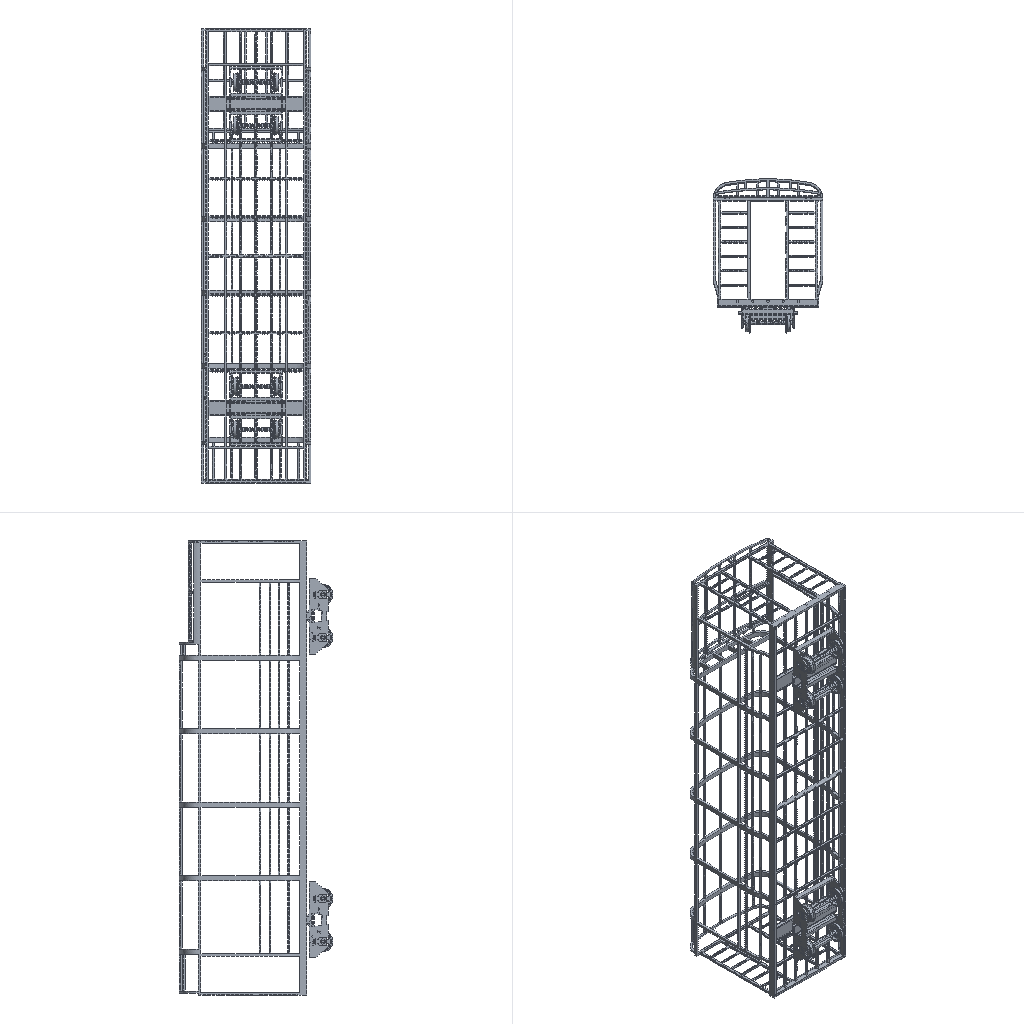Simulation study | ansys workbench
Set-up summary:
category,name,step,type,value,unit,region
solver,ansys_workbench
units,mm-N-s-tonne (MPa),,stated,"/units,MPA"
analysis,LS1,,static
load_step,LS1,LS1,static,nsubst=1; time=1
mesh,nodes,,,844921
mesh,elements,,,484857
element_type,SOLID187,,,440747
element_type,CONTA174,,,29118
element_type,TARGE170,,,10972
element_type,SOLID186,,,4020
material,Structural Steel,,E,200000,tonne s^-2 mm^-1
material,Structural Steel,,nu,0.3
material,Structural Steel,,density,7.85e-09,tonne mm^-3
material,Structural Steel,,conductivity,60.5,tonne mm s^-3 C^-1
material,Structural Steel,,specific_heat,4.34e+08,mm^2 s^-2 C^-1
material,Structural Steel,,cte,1.2e-05,C^-1
material,Structural Steel,,permeability,10000
material,Structural Steel,,resistivity,0.00017,ohm mm
load,,LS1,moment,"2.62e+06 [dir=(1, 0, 0) n=12]",,all
load,,LS1,force,"4284 [dir=(-1, 0, 0) n=3]",,all
load,ACEL,LS1,gravity (ACEL; gravity acts opposite),"9806.41 [dir=(0, 0.9996, 0.02998)]",,all
bc,Constant Zero Displacement X,model,fixed,[dofs=UX],,_DISPZEROUX
bc,Constant Zero Displacement Y,model,fixed,[dofs=UY],,_DISPZEROUY
bc,Constant Zero Displacement Z,model,fixed,[dofs=UZ],,_DISPZEROUZ
contact,Contact Region 10,,bonded (always),element=CONTA174
contact,Contact Region 11,,bonded (always),element=CONTA174
contact,Contact Region 12,,bonded (always),element=CONTA174
contact,Contact Region 13,,bonded (always),element=CONTA174
contact,Contact Region 14,,bonded (always),element=CONTA174
contact,Contact Region 15,,bonded (always),element=CONTA174
contact,Contact Region 16,,bonded (always),element=CONTA174
contact,Contact Region 17,,bonded (always),element=CONTA174
contact,Contact Region 18,,bonded (always),element=CONTA174
contact,Contact Region 19,,bonded (always),element=CONTA174
contact,Contact Region 20,,bonded (always),element=CONTA174
contact,Contact Region 21,,bonded (always),element=CONTA174
contact,Contact Region 22,,bonded (always),element=CONTA174
contact,Contact Region 23,,bonded (always),element=CONTA174
contact,Contact Region 24,,bonded (always),element=CONTA174
contact,Contact Region 25,,bonded (always),element=CONTA174
contact,Contact Region 26,,bonded (always),element=CONTA174
contact,Contact Region 27,,bonded (always),element=CONTA174
contact,Contact Region 28,,bonded (always),element=CONTA174
contact,Contact Region 29,,bonded (always),element=CONTA174
contact,Contact Region 30,,bonded (always),element=CONTA174
contact,Contact Region 31,,bonded (always),element=CONTA174
contact,Contact Region 32,,bonded (always),element=CONTA174
contact,Contact Region 33,,bonded (always),element=CONTA174
contact,Contact Region 34,,bonded (always),element=CONTA174
contact,Contact Region 35,,bonded (always),element=CONTA174
contact,Contact Region 36,,bonded (always),element=CONTA174
contact,Contact Region 37,,bonded (always),element=CONTA174
contact,Contact Region 38,,bonded (always),element=CONTA174
contact,Contact Region 39,,bonded (always),element=CONTA174
contact,Contact Region 40,,bonded (always),element=CONTA174
contact,Contact Region 41,,bonded (always),element=CONTA174
contact,Contact Region 42,,bonded (always),element=CONTA174
contact,Contact Region 43,,bonded (always),element=CONTA174
contact,Contact Region 44,,bonded (always),element=CONTA174
contact,Contact Region 45,,bonded (always),element=CONTA174
contact,Contact Region 46,,bonded (always),element=CONTA174
contact,Contact Region 47,,bonded (always),element=CONTA174
contact,Contact Region 48,,bonded (always),element=CONTA174
contact,Contact Region 49,,bonded (always),element=CONTA174
contact,Contact Region 50,,bonded (always),element=CONTA174
contact,Contact Region 51,,bonded (always),element=CONTA174
contact,Contact Region 52,,bonded (always),element=CONTA174
contact,Contact Region 53,,bonded (always),element=CONTA174
contact,Contact Region 54,,bonded (always),element=CONTA174
contact,Contact Region 55,,bonded (always),element=CONTA174
contact,Contact Region 56,,bonded (always),element=CONTA174
contact,Contact Region 57,,bonded (always),element=CONTA174
contact,Contact Region 58,,bonded (always),element=CONTA174
contact,Contact Region 59,,bonded (always),element=CONTA174
contact,Contact Region 60,,bonded (always),element=CONTA174
contact,Contact Region 61,,bonded (always),element=CONTA174
contact,Contact Region 62,,bonded (always),element=CONTA174
contact,Contact Region 63,,bonded (always),element=CONTA174
contact,Contact Region 64,,bonded (always),element=CONTA174
contact,Contact Region 65,,bonded (always),element=CONTA174
contact,Contact Region 66,,bonded (always),element=CONTA174
contact,Contact Region 67,,bonded (always),element=CONTA174
contact,Contact Region 68,,bonded (always),element=CONTA174
contact,Contact Region 69,,bonded (always),element=CONTA174
contact,Contact Region 70,,bonded (always),element=CONTA174
contact,Contact Region 71,,bonded (always),element=CONTA174
contact,Contact Region 72,,bonded (always),element=CONTA174
contact,Contact Region 73,,bonded (always),element=CONTA174
contact,Contact Region 74,,bonded (always),element=CONTA174
contact,Contact Region 75,,bonded (always),element=CONTA174
contact,Contact Region 76,,bonded (always),element=CONTA174
contact,Contact Region 77,,bonded (always),element=CONTA174
contact,Contact Region 78,,bonded (always),element=CONTA174
contact,Contact Region 79,,bonded (always),element=CONTA174
contact,Contact Region 80,,bonded (always),element=CONTA174
contact,Contact Region 81,,bonded (always),element=CONTA174
contact,Contact Region 82,,bonded (always),element=CONTA174
contact,Contact Region 83,,bonded (always),element=CONTA174
contact,Contact Region 84,,bonded (always),element=CONTA174
contact,Contact Region 85,,bonded (always),element=CONTA174
contact,Contact Region 86,,bonded (always),element=CONTA174
contact,Contact Region 87,,bonded (always),element=CONTA174
contact,Contact Region 88,,bonded (always),element=CONTA174
contact,Contact Region 89,,bonded (always),element=CONTA174
contact,Contact Region 90,,bonded (always),element=CONTA174
contact,Contact Region 91,,bonded (always),element=CONTA174
contact,Contact Region 92,,bonded (always),element=CONTA174
contact,Contact Region 93,,bonded (always),element=CONTA174
contact,Contact Region 94,,bonded (always),element=CONTA174
contact,Contact Region 95,,bonded (always),element=CONTA174
contact,Contact Region 96,,bonded (always),element=CONTA174
contact,Contact Region 97,,bonded (always),element=CONTA174
contact,Contact Region 98,,bonded (always),element=CONTA174
contact,Contact Region 99,,bonded (always),element=CONTA174
contact,Contact Region 100,,bonded (always),element=CONTA174
contact,Contact Region 101,,bonded (always),element=CONTA174
contact,Contact Region 102,,bonded (always),element=CONTA174
contact,Contact Region 103,,bonded (always),element=CONTA174
contact,Contact Region 104,,bonded (always),element=CONTA174
contact,Contact Region 105,,bonded (always),element=CONTA174
contact,Contact Region 106,,bonded (always),element=CONTA174
contact,Contact Region 107,,bonded (always),element=CONTA174
contact,Contact Region 108,,bonded (always),element=CONTA174
contact,Contact Region 109,,bonded (always),element=CONTA174
contact,Contact Region 110,,bonded (always),element=CONTA174
contact,Contact Region 111,,bonded (always),element=CONTA174
contact,Contact Region 112,,bonded (always),element=CONTA174
contact,Contact Region 113,,bonded (always),element=CONTA174
contact,Contact Region 114,,bonded (always),element=CONTA174
contact,Contact Region 115,,bonded (always),element=CONTA174
contact,Contact Region 116,,bonded (always),element=CONTA174
contact,Contact Region 117,,bonded (always),element=CONTA174
contact,Contact Region 118,,bonded (always),element=CONTA174
contact,Contact Region 119,,bonded (always),element=CONTA174
contact,Contact Region 120,,bonded (always),element=CONTA174
contact,contact 112,,bonded (always),element=CONTA174
contact,contact 113,,bonded (always),element=CONTA174
contact,contact 114,,bonded (always),element=CONTA174
contact,contact 115,,bonded (always),element=CONTA174
contact,contact 116,,bonded (always),element=CONTA174
contact,contact 117,,bonded (always),element=CONTA174
contact,contact 118,,bonded (always),element=CONTA174
named_set,_DISPZEROUX,,node,2976
named_set,_DISPZEROUY,,node,2976
named_set,_DISPZEROUZ,,node,1488
Ansys APDL input file, long lists of numbers shortened:
/batch
/config,noeldb,1     ! force off writing results to database
*get,_wallstrt,active,,time,wall
! ANSYS input file written by Workbench version 2021 R1
! File used for geometry attach:
/title,_______--____ (B5)
! ****** Begin Custom Load Command Snippet ******
/COM, ACT Extensions:
/COM,     LSDYNA, 2021.1
/COM,
! ****** End   Custom Load Command Snippet ******
*DIM,_wb_ProjectScratch_dir,string,248
_wb_ProjectScratch_dir(1) = ''
*DIM,_wb_SolverFiles_dir,string,248
_wb_SolverFiles_dir(1) = ''
*DIM,_wb_userfiles_dir,string,248
_wb_userfiles_dir(1) = ''
/com,--- Data in consistent NMM units. See Solving Units in the help system for more information.
/units,MPA
/nopr
/wb,file,start              !  signify a WB generated input file
/prep7
! Turn off shape checking because checks already performed inside WB mesher.
! See help system for more information.
SHPP,OFF,,NOWARN
/nolist
etcon,set             ! allow ANSYS to choose best KEYOP's for 180x elements, resets any applicable keyopt to MAPDL defaults
/com,*********** Nodes for the whole assembly ***********
nblock,3,,929390
(1i9,3e20.9e3)
        1     5.000000000E+02    -2.700000000E+02     8.500000000E+01
! (844899 more lines like these left out)
-1
/com,*********** Nodes for all Remote Points ***********
nblock,3
(1i9,3e20.9e3)
   844901     0.000000000E+00    -4.570000000E+02     1.250000000E+03
! (20 more lines like these left out)
-1
/wb,elem,start            !  set before creation of elements
/com,*********** Elements for Body 1 "____-0|NONE" ***********
et,1,187
eblock,19,solid,,219008
(19i9)
        1        1        1        1        0        0        0        0       10        0   225760   496373   499028   502293   501893   835194   841376   835201   835199
! (438015 more lines like these left out)
-1
/com,*********** Elements for Body 2 "______|NONE" ***********
et,2,186
keyo,2,2,1          ! set full integration on SOLID186
eblock,19,solid,,316
(19i9)
        2        2        2        2        0        0        0        0       20        0      914     6556     6586     6589     6565     6931     6901     6898     6922
! (631 more lines like these left out)
-1
/com,*********** Elements for Body 3 "______|NONE[2]" ***********
et,3,186
keyo,3,2,1          ! set full integration on SOLID186
eblock,19,solid,,316
(19i9)
        3        3        3        3        0        0        0        0       20        0     1663    12147    12177    12180    12156    12522    12492    12489    12513
! (631 more lines like these left out)
-1
/com,*********** Elements for Body 4 "______|NONE[3]" ***********
et,4,186
keyo,4,2,1          ! set full integration on SOLID186
eblock,19,solid,,420
(19i9)
        4        4        4        4        0        0        0        0       20        0     1243     9304     9447     9466     9364     9345     9446     9485     9365
! (839 more lines like these left out)
-1
/com,*********** Elements for Body 5 "______|NONE[4]" ***********
et,5,186
keyo,5,2,1          ! set full integration on SOLID186
eblock,19,solid,,420
(19i9)
        5        5        5        5        0        0        0        0       20        0      481     3579     3722     3741     3639     3620     3721     3760     3640
! (839 more lines like these left out)
-1
! (55 more sections like these left out)
/wb,elem,end               !  done creating elements
/com,*********** Send User Defined Coordinate System(s) ***********
csys,0
toffst,273.15,  ! Temperature offset from absolute zero
/com,*********** Set Reference Temperature ***********
tref,22.
/wb,mat,start              !  starting to send materials
/com,*********** Send Materials ***********
Temperature = 'TEMP' ! Temperature
MP,DENS,1,7.85e-09,	! tonne mm^-3
MP,ALPX,1,1.2e-05,	! C^-1
MP,C,1,434000000,	! mm^2 s^-2 C^-1
MP,KXX,1,60.5,	! tonne mm s^-3 C^-1
MP,RSVX,1,0.00017,	! ohm mm
MP,EX,1,200000,	! tonne s^-2 mm^-1
MP,NUXY,1,0.3,
MP,MURX,1,10000,
Temperature = 'TEMP' ! Temperature
MP,DENS,2,7.85e-09,	! tonne mm^-3
MP,ALPX,2,1.2e-05,	! C^-1
MP,C,2,434000000,	! mm^2 s^-2 C^-1
MP,KXX,2,60.5,	! tonne mm s^-3 C^-1
MP,RSVX,2,0.00017,	! ohm mm
MP,EX,2,200000,	! tonne s^-2 mm^-1
MP,NUXY,2,0.3,
MP,MURX,2,10000,
Temperature = 'TEMP' ! Temperature
MP,DENS,3,7.85e-09,	! tonne mm^-3
MP,ALPX,3,1.2e-05,	! C^-1
MP,C,3,434000000,	! mm^2 s^-2 C^-1
MP,KXX,3,60.5,	! tonne mm s^-3 C^-1
MP,RSVX,3,0.00017,	! ohm mm
MP,EX,3,200000,	! tonne s^-2 mm^-1
MP,NUXY,3,0.3,
MP,MURX,3,10000,
Temperature = 'TEMP' ! Temperature
MP,DENS,4,7.85e-09,	! tonne mm^-3
MP,ALPX,4,1.2e-05,	! C^-1
MP,C,4,434000000,	! mm^2 s^-2 C^-1
MP,KXX,4,60.5,	! tonne mm s^-3 C^-1
MP,RSVX,4,0.00017,	! ohm mm
MP,EX,4,200000,	! tonne s^-2 mm^-1
MP,NUXY,4,0.3,
MP,MURX,4,10000,
Temperature = 'TEMP' ! Temperature
MP,DENS,5,7.85e-09,	! tonne mm^-3
MP,ALPX,5,1.2e-05,	! C^-1
MP,C,5,434000000,	! mm^2 s^-2 C^-1
MP,KXX,5,60.5,	! tonne mm s^-3 C^-1
MP,RSVX,5,0.00017,	! ohm mm
MP,EX,5,200000,	! tonne s^-2 mm^-1
MP,NUXY,5,0.3,
MP,MURX,5,10000,
Temperature = 'TEMP' ! Temperature
MP,DENS,6,7.85e-09,	! tonne mm^-3
MP,ALPX,6,1.2e-05,	! C^-1
MP,C,6,434000000,	! mm^2 s^-2 C^-1
MP,KXX,6,60.5,	! tonne mm s^-3 C^-1
MP,RSVX,6,0.00017,	! ohm mm
MP,EX,6,200000,	! tonne s^-2 mm^-1
MP,NUXY,6,0.3,
MP,MURX,6,10000,
Temperature = 'TEMP' ! Temperature
MP,DENS,7,7.85e-09,	! tonne mm^-3
MP,ALPX,7,1.2e-05,	! C^-1
MP,C,7,434000000,	! mm^2 s^-2 C^-1
MP,KXX,7,60.5,	! tonne mm s^-3 C^-1
MP,RSVX,7,0.00017,	! ohm mm
MP,EX,7,200000,	! tonne s^-2 mm^-1
MP,NUXY,7,0.3,
MP,MURX,7,10000,
Temperature = 'TEMP' ! Temperature
MP,DENS,8,7.85e-09,	! tonne mm^-3
MP,ALPX,8,1.2e-05,	! C^-1
MP,C,8,434000000,	! mm^2 s^-2 C^-1
MP,KXX,8,60.5,	! tonne mm s^-3 C^-1
MP,RSVX,8,0.00017,	! ohm mm
MP,EX,8,200000,	! tonne s^-2 mm^-1
MP,NUXY,8,0.3,
MP,MURX,8,10000,
Temperature = 'TEMP' ! Temperature
MP,DENS,9,7.85e-09,	! tonne mm^-3
MP,ALPX,9,1.2e-05,	! C^-1
MP,C,9,434000000,	! mm^2 s^-2 C^-1
MP,KXX,9,60.5,	! tonne mm s^-3 C^-1
MP,RSVX,9,0.00017,	! ohm mm
MP,EX,9,200000,	! tonne s^-2 mm^-1
! (461 more lines like these left out)
/wb,mat,end                !  done sending materials
!************************* Model Summary ********************
!____-0|NONE,	结构钢,	matid,	1
!______|NONE,	结构钢,	matid,	2
!______|NONE[2],	结构钢,	matid,	3
! (59 more lines like these left out)
*get,_xmin,node,,mnloc,x
*get,_ymin,node,,mnloc,y
*get,_zmin,node,,mnloc,z
*get,_xmax,node,,mxloc,x
*get,_ymax,node,,mxloc,y
*get,_zmax,node,,mxloc,z
_ASMDIAG=(_xmax-_xmin)*(_xmax-_xmin)+(_ymax-_ymin)*(_ymax-_ymin)+(_zmax-_zmin)*(_zmax-_zmin)
_ASMDIAG=SQRT(_ASMDIAG)
/wb,contact,start          !  starting to send contact
/com,*********** Create Contact "接触区域 10" ***********
/com,            Real Constant Set For Above Contact Is 62 & 61
*set,tid,62
*set,cid,61
r,tid
r,cid
et,tid,170
et,cid,174
eblock,10,,,42
(15i9)
   662849       62       62       62        0     6714     6723     6734     6734     7990     8015     6734     7992
! (41 more lines like these left out)
-1
eblock,10,,,42
(15i9)
   662891       61       61       61        0     6714     6723     6734     6734     7990     8015     6734     7992
! (41 more lines like these left out)
-1
eblock,10,,,21
(15i9)
   662933       61       62       61        0     9885    10045     9244     9244    11813    10203     9244    10202
! (20 more lines like these left out)
-1
eblock,10,,,21
(15i9)
   662954       62       61       62        0     9885    10045     9244     9244    11813    10203     9244    10202
! (20 more lines like these left out)
-1
keyo,cid,8,2               ! auto create asymmetric contact (from Program Controlled setting)
keyo,cid,10,0              ! adjust contact stiffness each NR iteration (from Program Controlled setting)
keyo,cid,12,5              ! bonded always
keyo,cid,18,1              ! small sliding turned on by application
keyo,cid,2,0               ! augmented Lagrange (from Program Controlled setting)
keyo,cid,4,0               ! on Gauss point (from Program Controlled setting)
keyo,cid,9,1               ! ignore initial gaps/penetration
keyo,cid,7,0               ! No Prediction
rmod,tid,3,10.      ! FKN
rmod,tid,5,0.       ! ICONT
rmod,tid,6,0.       ! PINB
rmod,tid,10,0.      ! CNOF
rmod,tid,12,0.      ! FKT
rmod,tid,36,14962   ! WB DSID
rmod,cid,3,10.      ! FKN
rmod,cid,5,0.       ! ICONT
rmod,cid,6,0.       ! PINB
rmod,cid,10,0.      ! CNOF
rmod,cid,12,0.      ! FKT
rmod,cid,36,14962   ! WB DSID
/com,*********** Create Contact "接触区域 11" ***********
/com,            Real Constant Set For Above Contact Is 64 & 63
*set,tid,64
*set,cid,63
r,tid
r,cid
et,tid,170
et,cid,174
eblock,10,,,48
(15i9)
   662975       64       64       64        0     6688     6733     6595     6595     7938     7613     6595     7610
! (47 more lines like these left out)
-1
eblock,10,,,48
(15i9)
   663023       63       63       63        0     6688     6733     6595     6595     7938     7613     6595     7610
! (47 more lines like these left out)
-1
eblock,10,,,21
(15i9)
   663071       63       64       63        0     3534     3522     3523     3523     4485     4484     3523     4488
! (20 more lines like these left out)
-1
eblock,10,,,21
(15i9)
   663092       64       63       64        0     3534     3522     3523     3523     4485     4484     3523     4488
! (20 more lines like these left out)
-1
keyo,cid,8,2               ! auto create asymmetric contact (from Program Controlled setting)
keyo,cid,10,0              ! adjust contact stiffness each NR iteration (from Program Controlled setting)
keyo,cid,12,5              ! bonded always
keyo,cid,18,1              ! small sliding turned on by application
keyo,cid,2,0               ! augmented Lagrange (from Program Controlled setting)
keyo,cid,4,0               ! on Gauss point (from Program Controlled setting)
keyo,cid,9,1               ! ignore initial gaps/penetration
keyo,cid,7,0               ! No Prediction
rmod,tid,3,10.      ! FKN
rmod,tid,5,0.       ! ICONT
rmod,tid,6,0.       ! PINB
rmod,tid,10,0.      ! CNOF
rmod,tid,12,0.      ! FKT
rmod,tid,36,14965   ! WB DSID
rmod,cid,3,10.      ! FKN
rmod,cid,5,0.       ! ICONT
rmod,cid,6,0.       ! PINB
rmod,cid,10,0.      ! CNOF
rmod,cid,12,0.      ! FKT
rmod,cid,36,14965   ! WB DSID
/com,*********** Create Contact "接触区域 12" ***********
/com,            Real Constant Set For Above Contact Is 66 & 65
*set,tid,66
*set,cid,65
r,tid
r,cid
et,tid,170
et,cid,174
eblock,10,,,16
(15i9)
   663113       66       66       66        0     6741     6708     6696     6709     7977     7955     7956     7980
! (15 more lines like these left out)
-1
eblock,10,,,16
(15i9)
   663129       65       65       65        0     6741     6708     6696     6709     7977     7955     7956     7980
! (15 more lines like these left out)
-1
eblock,10,,,12
(15i9)
   663145       65       66       65        0     1744     1745     1761     1756     2255     2259     2289     2257
! (11 more lines like these left out)
-1
eblock,10,,,12
(15i9)
   663157       66       65       66        0     1744     1745     1761     1756     2255     2259     2289     2257
! (11 more lines like these left out)
-1
keyo,cid,8,2               ! auto create asymmetric contact (from Program Controlled setting)
keyo,cid,10,0              ! adjust contact stiffness each NR iteration (from Program Controlled setting)
keyo,cid,12,5              ! bonded always
keyo,cid,18,1              ! small sliding turned on by application
keyo,cid,2,0               ! augmented Lagrange (from Program Controlled setting)
keyo,cid,4,0               ! on Gauss point (from Program Controlled setting)
keyo,cid,9,1               ! ignore initial gaps/penetration
keyo,cid,7,0               ! No Prediction
rmod,tid,3,10.      ! FKN
rmod,tid,5,0.       ! ICONT
rmod,tid,6,0.       ! PINB
rmod,tid,10,0.      ! CNOF
rmod,tid,12,0.      ! FKT
rmod,tid,36,14968   ! WB DSID
rmod,cid,3,10.      ! FKN
rmod,cid,5,0.       ! ICONT
rmod,cid,6,0.       ! PINB
rmod,cid,10,0.      ! CNOF
rmod,cid,12,0.      ! FKT
rmod,cid,36,14968   ! WB DSID
/com,*********** Create Contact "接触区域 13" ***********
/com,            Real Constant Set For Above Contact Is 68 & 67
*set,tid,68
*set,cid,67
r,tid
r,cid
et,tid,170
et,cid,174
eblock,10,,,15
(15i9)
   663169       68       68       68        0     6738     6691     6692     6739     7945     7944     7948     8042
! (14 more lines like these left out)
-1
eblock,10,,,15
(15i9)
   663184       67       67       67        0     6738     6691     6692     6739     7945     7944     7948     8042
! (14 more lines like these left out)
-1
eblock,10,,,12
(15i9)
   663199       67       68       67        0       21       16        4        5      549      517      515      519
! (11 more lines like these left out)
-1
eblock,10,,,12
(15i9)
   663211       68       67       68        0       21       16        4        5      549      517      515      519
! (11 more lines like these left out)
-1
keyo,cid,8,2               ! auto create asymmetric contact (from Program Controlled setting)
keyo,cid,10,0              ! adjust contact stiffness each NR iteration (from Program Controlled setting)
keyo,cid,12,5              ! bonded always
keyo,cid,18,1              ! small sliding turned on by application
keyo,cid,2,0               ! augmented Lagrange (from Program Controlled setting)
keyo,cid,4,0               ! on Gauss point (from Program Controlled setting)
keyo,cid,9,1               ! ignore initial gaps/penetration
keyo,cid,7,0               ! No Prediction
rmod,tid,3,10.      ! FKN
rmod,tid,5,0.       ! ICONT
rmod,tid,6,0.       ! PINB
rmod,tid,10,0.      ! CNOF
rmod,tid,12,0.      ! FKT
rmod,tid,36,14971   ! WB DSID
rmod,cid,3,10.      ! FKN
rmod,cid,5,0.       ! ICONT
rmod,cid,6,0.       ! PINB
rmod,cid,10,0.      ! CNOF
rmod,cid,12,0.      ! FKT
rmod,cid,36,14971   ! WB DSID
/com,*********** Create Contact "接触区域 14" ***********
/com,            Real Constant Set For Above Contact Is 70 & 69
*set,tid,70
*set,cid,69
r,tid
r,cid
et,tid,170
et,cid,174
eblock,10,,,33
(15i9)
   663223       70       70       70        0     7129     7127     7128     7133     8908     8907     8909     8911
! (32 more lines like these left out)
-1
eblock,10,,,33
(15i9)
   663256       69       69       69        0     7129     7127     7128     7133     8908     8907     8909     8911
! (32 more lines like these left out)
-1
eblock,10,,,170
(15i9)
   663289       69       70       69        0    17468    17488    17473    17473    26290    26306    17473    26287
! (169 more lines like these left out)
-1
eblock,10,,,170
(15i9)
   663459       70       69       70        0    17468    17488    17473    17473    26290    26306    17473    26287
! (169 more lines like these left out)
-1
keyo,cid,8,2               ! auto create asymmetric contact (from Program Controlled setting)
keyo,cid,10,0              ! adjust contact stiffness each NR iteration (from Program Controlled setting)
keyo,cid,12,5              ! bonded always
keyo,cid,18,1              ! small sliding turned on by application
keyo,cid,2,0               ! augmented Lagrange (from Program Controlled setting)
keyo,cid,4,0               ! on Gauss point (from Program Controlled setting)
keyo,cid,9,1               ! ignore initial gaps/penetration
keyo,cid,7,0               ! No Prediction
rmod,tid,3,10.      ! FKN
rmod,tid,5,0.       ! ICONT
rmod,tid,6,0.       ! PINB
rmod,tid,10,0.      ! CNOF
rmod,tid,12,0.      ! FKT
rmod,tid,36,14974   ! WB DSID
rmod,cid,3,10.      ! FKN
rmod,cid,5,0.       ! ICONT
rmod,cid,6,0.       ! PINB
rmod,cid,10,0.      ! CNOF
rmod,cid,12,0.      ! FKT
rmod,cid,36,14974   ! WB DSID
! (106 more sections like these left out)
/wb,contact,end            !  done creating contacts
/golist
/wb,load,start             !  starting to send loads
/com,******* Constant Zero Displacement X *******
CMBLOCK,_DISPZEROUX,NODE,     2976
(8i10)
     33525     33526     33527     33528     33529     33530     33531     33532
! (371 more lines like these left out)
cmsel,s,_DISPZEROUX
d,all,ux,0
nsel,all
/com,******* Constant Zero Displacement Y *******
CMBLOCK,_DISPZEROUY,NODE,     2976
(8i10)
     33525     33526     33527     33528     33529     33530     33531     33532
! (371 more lines like these left out)
cmsel,s,_DISPZEROUY
d,all,uy,0
nsel,all
/com,******* Constant Zero Displacement Z *******
CMBLOCK,_DISPZEROUZ,NODE,     1488
(8i10)
     33525     33526     33527     33528     33529     33530     33531     33532
! (185 more lines like these left out)
cmsel,s,_DISPZEROUZ
d,all,uz,0
nsel,all
/com,*********** Create Remote Point "内部远程点" ***********
! -------- Remote Point Used by "力矩" --------
*set,tid,284
*set,cid,283
et,cid,174
et,tid,170
keyo,tid,2,1               ! Don't fix the pilot node
keyo,tid,4,0               ! Activate all DOF's due to large deformation
keyo,cid,12,5              ! Bonded Contact
keyo,cid,4,1               ! Deformable RBE3 style load
keyo,cid,2,2               ! MPC style contact
eblock,10,,,358
(15i9)
   684793      283      283      283        0    38713    38614    38728    38728    39254    39255    38728    40038
! (357 more lines like these left out)
-1
*set,_npilot,844901
_npilot12361=_npilot
type,tid
mat ,cid
real,cid
tshape,pilo
en,685151,_npilot
tshape
/com,*********** Create Remote Point "内部远程点 2" ***********
! -------- Remote Point Used by "力矩 2" --------
*set,tid,286
*set,cid,285
et,cid,174
et,tid,170
keyo,tid,2,1               ! Don't fix the pilot node
keyo,tid,4,0               ! Activate all DOF's due to large deformation
keyo,cid,12,5              ! Bonded Contact
keyo,cid,4,1               ! Deformable RBE3 style load
keyo,cid,2,2               ! MPC style contact
eblock,10,,,360
(15i9)
   685152      285      285      285        0    71272    71189    71399    71399    72063    72066    71399    72735
! (359 more lines like these left out)
-1
*set,_npilot,844902
_npilot12364=_npilot
type,tid
mat ,cid
real,cid
tshape,pilo
en,685512,_npilot
tshape
/com,*********** Create Remote Point "内部远程点 3" ***********
! -------- Remote Point Used by "力矩 3" --------
*set,tid,288
*set,cid,287
et,cid,174
et,tid,170
keyo,tid,2,1               ! Don't fix the pilot node
keyo,tid,4,0               ! Activate all DOF's due to large deformation
keyo,cid,12,5              ! Bonded Contact
keyo,cid,4,1               ! Deformable RBE3 style load
keyo,cid,2,2               ! MPC style contact
eblock,10,,,358
(15i9)
   685513      287      287      287        0    27853    27754    27868    27868    28394    28395    27868    29178
! (357 more lines like these left out)
-1
*set,_npilot,844903
_npilot12367=_npilot
type,tid
mat ,cid
real,cid
tshape,pilo
en,685871,_npilot
tshape
/com,*********** Create Remote Point "内部远程点 4" ***********
! -------- Remote Point Used by "力矩 4" --------
*set,tid,290
*set,cid,289
et,cid,174
et,tid,170
keyo,tid,2,1               ! Don't fix the pilot node
keyo,tid,4,0               ! Activate all DOF's due to large deformation
keyo,cid,12,5              ! Bonded Contact
keyo,cid,4,1               ! Deformable RBE3 style load
keyo,cid,2,2               ! MPC style contact
eblock,10,,,360
(15i9)
   685872      289      289      289        0    60036    59953    60163    60163    60827    60830    60163    61499
! (359 more lines like these left out)
-1
*set,_npilot,844904
_npilot12370=_npilot
type,tid
mat ,cid
real,cid
tshape,pilo
en,686232,_npilot
tshape
/com,*********** Create Remote Point "内部远程点 17" ***********
! -------- Remote Point Used by "乘客重量" --------
*set,tid,292
*set,cid,291
et,cid,174
et,tid,170
keyo,tid,2,1               ! Don't fix the pilot node
keyo,tid,4,0               ! Activate all DOF's due to large deformation
keyo,cid,12,5              ! Bonded Contact
keyo,cid,4,1               ! Deformable RBE3 style load
keyo,cid,2,2               ! MPC style contact
eblock,10,,,6072
(15i9)
   686233      291      291      291        0   148608   149004   149355   149355   346755   349666   149355   346758
! (6071 more lines like these left out)
-1
*set,_npilot,844917
_npilot15533=_npilot
type,tid
mat ,cid
real,cid
tshape,pilo
en,692305,_npilot
tshape
! (2 more sections like these left out)
/com,*********** Construct Moment Using Remote Attachment ***********
/com,*********** Construct Moment Using Remote Attachment ***********
*DIM,_loadvari12363x,TABLE,2,1,1,TIME,
! Time values
_loadvari12363x(1,0,1) = 0.
_loadvari12363x(2,0,1) = 1.
! Load values
_loadvari12363x(1,1,1) = 0.
_loadvari12363x(2,1,1) = 655000.
*DIM,_loadvari12363y,TABLE,2,1,1,TIME,
! Time values
_loadvari12363y(1,0,1) = 0.
_loadvari12363y(2,0,1) = 1.
! Load values
_loadvari12363y(1,1,1) = 0.
_loadvari12363y(2,1,1) = 0.
*DIM,_loadvari12363z,TABLE,2,1,1,TIME,
! Time values
_loadvari12363z(1,0,1) = 0.
_loadvari12363z(2,0,1) = 1.
! Load values
_loadvari12363z(1,1,1) = 0.
_loadvari12363z(2,1,1) = 0.
/com,*********** Construct Moment Using Remote Attachment ***********
*DIM,_loadvari12366x,TABLE,2,1,1,TIME,
! Time values
_loadvari12366x(1,0,1) = 0.
_loadvari12366x(2,0,1) = 1.
! Load values
_loadvari12366x(1,1,1) = 0.
_loadvari12366x(2,1,1) = 655000.
*DIM,_loadvari12366y,TABLE,2,1,1,TIME,
! Time values
_loadvari12366y(1,0,1) = 0.
_loadvari12366y(2,0,1) = 1.
! Load values
_loadvari12366y(1,1,1) = 0.
_loadvari12366y(2,1,1) = 0.
*DIM,_loadvari12366z,TABLE,2,1,1,TIME,
! Time values
_loadvari12366z(1,0,1) = 0.
_loadvari12366z(2,0,1) = 1.
! Load values
_loadvari12366z(1,1,1) = 0.
_loadvari12366z(2,1,1) = 0.
/com,*********** Construct Moment Using Remote Attachment ***********
*DIM,_loadvari12369x,TABLE,2,1,1,TIME,
! Time values
_loadvari12369x(1,0,1) = 0.
_loadvari12369x(2,0,1) = 1.
! Load values
_loadvari12369x(1,1,1) = 0.
_loadvari12369x(2,1,1) = 655000.
*DIM,_loadvari12369y,TABLE,2,1,1,TIME,
! Time values
_loadvari12369y(1,0,1) = 0.
_loadvari12369y(2,0,1) = 1.
! Load values
_loadvari12369y(1,1,1) = 0.
_loadvari12369y(2,1,1) = 0.
*DIM,_loadvari12369z,TABLE,2,1,1,TIME,
! Time values
_loadvari12369z(1,0,1) = 0.
_loadvari12369z(2,0,1) = 1.
! Load values
_loadvari12369z(1,1,1) = 0.
_loadvari12369z(2,1,1) = 0.
/com,*********** Construct Remote Force ***********
*DIM,_loadvari15584x,TABLE,2,1,1,TIME,
! Time values
_loadvari15584x(1,0,1) = 0.
_loadvari15584x(2,0,1) = 1.
! Load values
_loadvari15584x(1,1,1) = 0.
_loadvari15584x(2,1,1) = -4284.
*DIM,_loadvari15584y,TABLE,2,1,1,TIME,
! Time values
_loadvari15584y(1,0,1) = 0.
_loadvari15584y(2,0,1) = 1.
! Load values
_loadvari15584y(1,1,1) = 0.
_loadvari15584y(2,1,1) = 0.
*DIM,_loadvari15584z,TABLE,2,1,1,TIME,
! Time values
_loadvari15584z(1,0,1) = 0.
_loadvari15584z(2,0,1) = 1.
! Load values
_loadvari15584z(1,1,1) = 0.
_loadvari15584z(2,1,1) = 0.
/com,*********** Construct Remote Mass Using Remote Attachment ***********
*set,_tid,297
et,_tid,21           ! MASS21 element
type,_tid
mat ,_tid
real,_tid
keyo,_tid,3,2        ! 3d mass without rotary inertia
r,_tid,2.8
en,702946,844917
/com,*********** Construct Remote Mass Using Remote Attachment ***********
*set,_tid,298
et,_tid,21           ! MASS21 element
type,_tid
mat ,_tid
real,_tid
keyo,_tid,3,2        ! 3d mass without rotary inertia
r,_tid,0.45
en,702947,844918
/gst,on,on
fini
*get,_numnode,node,0,count
*get,_numelem,elem,0,count
*get, _MAXELEMNUM, elem, 0, NUM, MAX
*get, _MAXNODENUM, node, 0, NUM, MAX
*get, _MAXELEMTYPE, etyp, 0, NUM, MAX
*get, _MAXREALCONST, real, 0, NUM, MAX
/go
/wb,load,end               !  done creating loads
/com,--- Number of total nodes = %_numnode%
/com,--- Number of contact elements = 40090
/com,--- Number of spring elements = 0
/com,--- Number of bearing elements = 0
/com,--- Number of solid elements = 444767
/com,--- Number of condensed parts = 0
/com,--- Number of total elements = %_numelem%
*get,_wallbsol,active,,time,wall
/com,****************************************************************************
/com,*************************    SOLUTION       ********************************
/com,****************************************************************************
/solu
antype,0                   ! static analysis
nlgeom,on                  ! Turn on Large Deformation Effects
_thickRatio=0.1     ! Ratio of thick parts in the model
eqsl,sparse,,,,,1
cntr,print,1               ! print out contact info and also make no initial contact an error
cntr,out,yes               ! write contact output to file.cmn due to many contact pairs present
dmpoption,emat,no             ! Don't combine emat file for DANSYS
dmpoption,esav,no             ! Don't combine esav file for DANSYS
nldiag,cont,iter           ! print out contact info each equilibrium iteration
rescontrol,define,last,last,,dele	   ! Program Controlled
/com,****************************************************
/com,******************* SOLVE FOR LS 1 OF 1 ****************
nsel,s,node,,844901
f,all,mx,655000.
f,all,my,0.
f,all,mz,0.
nsel,s,node,,844902
f,all,mx,%_loadvari12363x%
f,all,my,%_loadvari12363y%
f,all,mz,%_loadvari12363z%
nsel,s,node,,844903
f,all,mx,%_loadvari12366x%
f,all,my,%_loadvari12366y%
f,all,mz,%_loadvari12366z%
nsel,s,node,,844904
f,all,mx,%_loadvari12369x%
f,all,my,%_loadvari12369y%
f,all,mz,%_loadvari12369z%
nsel,all
nsel,s,node,,844919
f,all,fx,%_loadvari15584x%
f,all,fy,%_loadvari15584y%
f,all,fz,%_loadvari15584z%
nsel,all
acel,0.,-9802.,-294.
/nopr
/gopr
/nolist
autots,on                  ! Workbench Program Controlled automatic time stepping
nsub,1,10,1                ! due to presence of general nonlinear
time,1.
outres,erase
outres,all,none
outres,nsol,all,
outres,rsol,all
outres,eangl,all
outres,etmp,all
outres,veng,all
outres,strs,all,
outres,epel,all,
outres,eppl,all,
outres,cont,all,
! *********** WB SOLVE COMMAND ***********
! check interactive state
*get,ANSINTER_,active,,int
*if,ANSINTER_,ne,0,then
/eof
*endif
solve
/com *************** Write FE CONNECTORS *********
CEWRITE,file,ce,,INTE
/com,****************************************************
/com,*************** FINISHED SOLVE FOR LS 1 *************
*get,_wallasol,active,,time,wall
/nopr
*get,_numnode,node,0,count
*get,_numelem,elem,0,count
*get, _MAXELEMNUM, elem, 0, NUM, MAX
*get, _MAXNODENUM, node, 0, NUM, MAX,,,INTERNAL
*get, _MAXELEMTYPE, etyp, 0, NUM, MAX
*get, _MAXREALCONST, real, 0, NUM, MAX
/gopr
/post1
xmlo,ENCODING,ISO-8859-1
xmlo,parm
/xml,parm,xml
fini
/gopr
*get,_walldone,active,,time,wall
_preptime=(_wallbsol-_wallstrt)*3600
_solvtime=(_wallasol-_wallbsol)*3600
_posttime=(_walldone-_wallasol)*3600
_totaltim=(_walldone-_wallstrt)*3600
*get,_dlbratio,active,0,solu,dlbr
*get,_combtime,active,0,solu,comb
/com,--- Total number of nodes = %_numnode%
/com,--- Total number of elements = %_numelem%
/com,--- Element load balance ratio = %_dlbratio%
/com,--- Time to combine distributed files = %_combtime%
/wb,file,end               ! done with WB generated input
Results summary:
result,analyses[0].index,,,1
result,analyses[0].system,,,SYS-1
result,analyses[0].deck,,,deck.dat
result,analyses[0].solve_status,,,completed
result,analyses[0].analysis_type,,,static
result,analyses[0].physics,,,mechanical
result,analyses[0].unit_system,,,"NMM: mm, ton, N, s, mV, mA, degC"
result,analyses[0].n_sets,,,1
result,analyses[0].load_steps[0].set,set=1,,1
result,analyses[0].load_steps[0].time_or_freq,set=1,,1
result,analyses[0].load_steps[0].max_displacement_magnitude,set=1,,4.008
result,analyses[0].load_steps[0].max_von_mises_nodal,set=1,,157.506
result,analyses[0].load_steps[0].reaction_force_sum_xyz[1],set=1,,4284
result,analyses[0].load_steps[0].reaction_force_sum_xyz[2],set=1,,-96329.9
result,analyses[0].load_steps[0].reaction_force_sum_xyz[3],set=1,,-2889.27
result,geometry_export[0][0],,,.step
result,geometry_export[0][1],,,ok
result,geometry_export[0][2],,,329